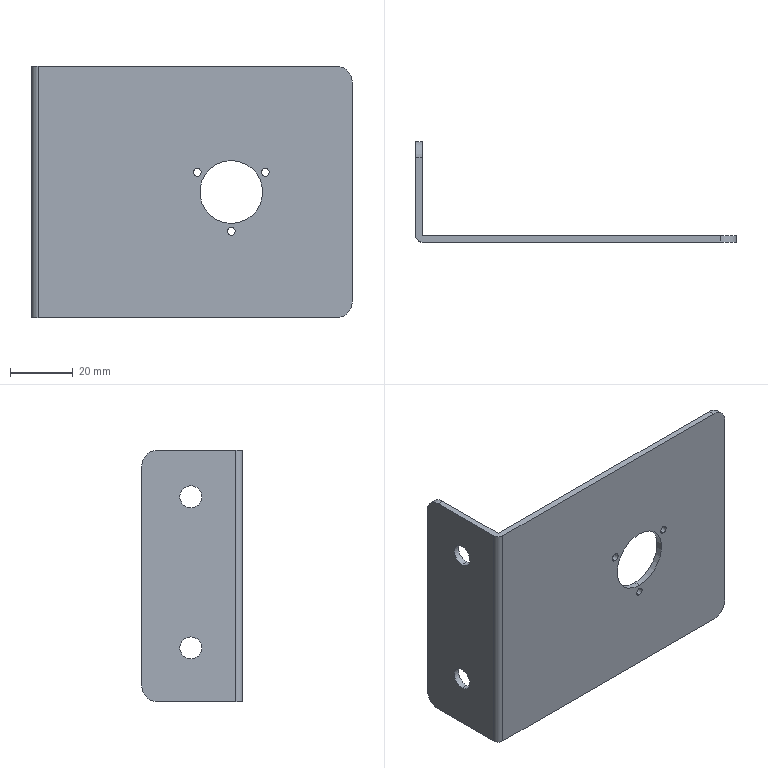Part | STEP file | 400v80 Rear Panel Filler Piece | 1 solid | 26 faces | box 102 x 32 x 80 mm | volume 20190 mm3 | cylinder 18 | plane 8 | commonest cylinder face diameters 2.5 x6 7 x4 10 x4 20 x2 0.2 x1 4.2 x1
STEP:
#1=CARTESIAN_POINT('',(39.258,-59.578,50.));
#2=VERTEX_POINT('',#1);
#3=CARTESIAN_POINT('',(39.258,-59.578,30.));
#4=VERTEX_POINT('',#3);
#5=CARTESIAN_POINT('',(39.258,-59.578,40.));
#6=DIRECTION('',(0.,-1.,0.));
#7=DIRECTION('',(0.,0.,1.));
#8=AXIS2_PLACEMENT_3D('',#5,#6,#7);
#9=CIRCLE('',#8,10.);
#10=EDGE_CURVE('',#2,#4,#9,.T.);
#11=ORIENTED_EDGE('',*,*,#10,.T.);
#12=CARTESIAN_POINT('',(39.258,-57.578,30.));
#13=VERTEX_POINT('',#12);
#14=CARTESIAN_POINT('',(39.258,-67.578,30.));
#15=DIRECTION('',(0.,1.,0.));
#16=VECTOR('',#15,1000.);
#17=LINE('',#14,#16);
#18=EDGE_CURVE('',#4,#13,#17,.T.);
#19=ORIENTED_EDGE('',*,*,#18,.T.);
#20=CARTESIAN_POINT('',(39.258,-57.578,50.));
#21=VERTEX_POINT('',#20);
#22=CARTESIAN_POINT('',(39.258,-57.578,40.));
#23=DIRECTION('',(0.,-1.,0.));
#24=DIRECTION('',(0.,0.,1.));
#25=AXIS2_PLACEMENT_3D('',#22,#23,#24);
#26=CIRCLE('',#25,10.);
#27=EDGE_CURVE('',#21,#13,#26,.T.);
#28=ORIENTED_EDGE('',*,*,#27,.F.);
#29=CARTESIAN_POINT('',(39.258,-67.578,50.));
#30=DIRECTION('',(0.,1.,0.));
#31=VECTOR('',#30,1000.);
#32=LINE('',#29,#31);
#33=EDGE_CURVE('',#2,#21,#32,.T.);
#34=ORIENTED_EDGE('',*,*,#33,.F.);
#35=EDGE_LOOP('',(#11,#19,#28,#34));
#36=FACE_OUTER_BOUND('',#35,.T.);
#37=CARTESIAN_POINT('',(39.258,-67.578,40.));
#38=DIRECTION('',(0.,1.,0.));
#39=DIRECTION('',(0.,0.,1.));
#40=AXIS2_PLACEMENT_3D('',#37,#38,#39);
#41=CYLINDRICAL_SURFACE('',#40,10.);
#42=ADVANCED_FACE('',(#36),#41,.F.);
#43=CARTESIAN_POINT('',(39.258,-59.578,28.75));
#44=VERTEX_POINT('',#43);
#45=CARTESIAN_POINT('',(39.258,-59.578,26.25));
#46=VERTEX_POINT('',#45);
#47=CARTESIAN_POINT('',(39.258,-59.578,27.5));
#48=DIRECTION('',(0.,-1.,0.));
#49=DIRECTION('',(0.,0.,1.));
#50=AXIS2_PLACEMENT_3D('',#47,#48,#49);
#51=CIRCLE('',#50,1.25);
#52=EDGE_CURVE('',#44,#46,#51,.T.);
#53=ORIENTED_EDGE('',*,*,#52,.T.);
#54=CARTESIAN_POINT('',(39.258,-57.578,26.25));
#55=VERTEX_POINT('',#54);
#56=CARTESIAN_POINT('',(39.258,-67.578,26.25));
#57=DIRECTION('',(0.,1.,0.));
#58=VECTOR('',#57,1000.);
#59=LINE('',#56,#58);
#60=EDGE_CURVE('',#46,#55,#59,.T.);
#61=ORIENTED_EDGE('',*,*,#60,.T.);
#62=CARTESIAN_POINT('',(39.258,-57.578,28.75));
#63=VERTEX_POINT('',#62);
#64=CARTESIAN_POINT('',(39.258,-57.578,27.5));
#65=DIRECTION('',(0.,-1.,0.));
#66=DIRECTION('',(0.,0.,1.));
#67=AXIS2_PLACEMENT_3D('',#64,#65,#66);
#68=CIRCLE('',#67,1.25);
#69=EDGE_CURVE('',#63,#55,#68,.T.);
#70=ORIENTED_EDGE('',*,*,#69,.F.);
#71=CARTESIAN_POINT('',(39.258,-67.578,28.75));
#72=DIRECTION('',(0.,1.,0.));
#73=VECTOR('',#72,1000.);
#74=LINE('',#71,#73);
#75=EDGE_CURVE('',#44,#63,#74,.T.);
#76=ORIENTED_EDGE('',*,*,#75,.F.);
#77=EDGE_LOOP('',(#53,#61,#70,#76));
#78=FACE_OUTER_BOUND('',#77,.T.);
#79=CARTESIAN_POINT('',(39.258,-67.578,27.5));
#80=DIRECTION('',(0.,1.,0.));
#81=DIRECTION('',(0.,0.,1.));
#82=AXIS2_PLACEMENT_3D('',#79,#80,#81);
#83=CYLINDRICAL_SURFACE('',#82,1.25);
#84=ADVANCED_FACE('',(#78),#83,.F.);
#85=CARTESIAN_POINT('',(50.084,-59.578,47.5));
#86=VERTEX_POINT('',#85);
#87=CARTESIAN_POINT('',(50.084,-59.578,45.));
#88=VERTEX_POINT('',#87);
#89=CARTESIAN_POINT('',(50.084,-59.578,46.25));
#90=DIRECTION('',(0.,-1.,0.));
#91=DIRECTION('',(0.,0.,1.));
#92=AXIS2_PLACEMENT_3D('',#89,#90,#91);
#93=CIRCLE('',#92,1.25);
#94=EDGE_CURVE('',#86,#88,#93,.T.);
#95=ORIENTED_EDGE('',*,*,#94,.T.);
#96=CARTESIAN_POINT('',(50.084,-57.578,45.));
#97=VERTEX_POINT('',#96);
#98=CARTESIAN_POINT('',(50.084,-67.578,45.));
#99=DIRECTION('',(0.,1.,0.));
#100=VECTOR('',#99,1000.);
#101=LINE('',#98,#100);
#102=EDGE_CURVE('',#88,#97,#101,.T.);
#103=ORIENTED_EDGE('',*,*,#102,.T.);
#104=CARTESIAN_POINT('',(50.084,-57.578,47.5));
#105=VERTEX_POINT('',#104);
#106=CARTESIAN_POINT('',(50.084,-57.578,46.25));
#107=DIRECTION('',(0.,-1.,0.));
#108=DIRECTION('',(0.,0.,1.));
#109=AXIS2_PLACEMENT_3D('',#106,#107,#108);
#110=CIRCLE('',#109,1.25);
#111=EDGE_CURVE('',#105,#97,#110,.T.);
#112=ORIENTED_EDGE('',*,*,#111,.F.);
#113=CARTESIAN_POINT('',(50.084,-67.578,47.5));
#114=DIRECTION('',(0.,1.,0.));
#115=VECTOR('',#114,1000.);
#116=LINE('',#113,#115);
#117=EDGE_CURVE('',#86,#105,#116,.T.);
#118=ORIENTED_EDGE('',*,*,#117,.F.);
#119=EDGE_LOOP('',(#95,#103,#112,#118));
#120=FACE_OUTER_BOUND('',#119,.T.);
#121=CARTESIAN_POINT('',(50.084,-67.578,46.25));
#122=DIRECTION('',(0.,1.,0.));
#123=DIRECTION('',(0.,0.,1.));
#124=AXIS2_PLACEMENT_3D('',#121,#122,#123);
#125=CYLINDRICAL_SURFACE('',#124,1.25);
#126=ADVANCED_FACE('',(#120),#125,.F.);
#127=CARTESIAN_POINT('',(28.433,-59.578,47.5));
#128=VERTEX_POINT('',#127);
#129=CARTESIAN_POINT('',(28.433,-59.578,45.));
#130=VERTEX_POINT('',#129);
#131=CARTESIAN_POINT('',(28.433,-59.578,46.25));
#132=DIRECTION('',(0.,-1.,0.));
#133=DIRECTION('',(0.,0.,1.));
#134=AXIS2_PLACEMENT_3D('',#131,#132,#133);
#135=CIRCLE('',#134,1.25);
#136=EDGE_CURVE('',#128,#130,#135,.T.);
#137=ORIENTED_EDGE('',*,*,#136,.T.);
#138=CARTESIAN_POINT('',(28.433,-57.578,45.));
#139=VERTEX_POINT('',#138);
#140=CARTESIAN_POINT('',(28.433,-67.578,45.));
#141=DIRECTION('',(0.,1.,0.));
#142=VECTOR('',#141,1000.);
#143=LINE('',#140,#142);
#144=EDGE_CURVE('',#130,#139,#143,.T.);
#145=ORIENTED_EDGE('',*,*,#144,.T.);
#146=CARTESIAN_POINT('',(28.433,-57.578,47.5));
#147=VERTEX_POINT('',#146);
#148=CARTESIAN_POINT('',(28.433,-57.578,46.25));
#149=DIRECTION('',(0.,-1.,0.));
#150=DIRECTION('',(0.,0.,1.));
#151=AXIS2_PLACEMENT_3D('',#148,#149,#150);
#152=CIRCLE('',#151,1.25);
#153=EDGE_CURVE('',#147,#139,#152,.T.);
#154=ORIENTED_EDGE('',*,*,#153,.F.);
#155=CARTESIAN_POINT('',(28.433,-67.578,47.5));
#156=DIRECTION('',(0.,1.,0.));
#157=VECTOR('',#156,1000.);
#158=LINE('',#155,#157);
#159=EDGE_CURVE('',#128,#147,#158,.T.);
#160=ORIENTED_EDGE('',*,*,#159,.F.);
#161=EDGE_LOOP('',(#137,#145,#154,#160));
#162=FACE_OUTER_BOUND('',#161,.T.);
#163=CARTESIAN_POINT('',(28.433,-67.578,46.25));
#164=DIRECTION('',(0.,1.,0.));
#165=DIRECTION('',(0.,0.,1.));
#166=AXIS2_PLACEMENT_3D('',#163,#164,#165);
#167=CYLINDRICAL_SURFACE('',#166,1.25);
#168=ADVANCED_FACE('',(#162),#167,.F.);
#169=CARTESIAN_POINT('',(-24.244,-43.225,61.712));
#170=VERTEX_POINT('',#169);
#171=CARTESIAN_POINT('',(-24.244,-43.225,68.712));
#172=VERTEX_POINT('',#171);
#173=CARTESIAN_POINT('',(-24.244,-43.225,65.212));
#174=DIRECTION('',(-1.,0.,0.));
#175=DIRECTION('',(0.,0.,-1.));
#176=AXIS2_PLACEMENT_3D('',#173,#174,#175);
#177=CIRCLE('',#176,3.5);
#178=EDGE_CURVE('',#170,#172,#177,.T.);
#179=ORIENTED_EDGE('',*,*,#178,.T.);
#180=CARTESIAN_POINT('',(-22.244,-43.225,68.712));
#181=VERTEX_POINT('',#180);
#182=CARTESIAN_POINT('',(-32.244,-43.225,68.712));
#183=DIRECTION('',(1.,0.,0.));
#184=VECTOR('',#183,1000.);
#185=LINE('',#182,#184);
#186=EDGE_CURVE('',#172,#181,#185,.T.);
#187=ORIENTED_EDGE('',*,*,#186,.T.);
#188=CARTESIAN_POINT('',(-22.244,-43.225,61.712));
#189=VERTEX_POINT('',#188);
#190=CARTESIAN_POINT('',(-22.244,-43.225,65.212));
#191=DIRECTION('',(-1.,0.,0.));
#192=DIRECTION('',(0.,0.,-1.));
#193=AXIS2_PLACEMENT_3D('',#190,#191,#192);
#194=CIRCLE('',#193,3.5);
#195=EDGE_CURVE('',#189,#181,#194,.T.);
#196=ORIENTED_EDGE('',*,*,#195,.F.);
#197=CARTESIAN_POINT('',(-32.244,-43.225,61.712));
#198=DIRECTION('',(1.,0.,0.));
#199=VECTOR('',#198,1000.);
#200=LINE('',#197,#199);
#201=EDGE_CURVE('',#170,#189,#200,.T.);
#202=ORIENTED_EDGE('',*,*,#201,.F.);
#203=EDGE_LOOP('',(#179,#187,#196,#202));
#204=FACE_OUTER_BOUND('',#203,.T.);
#205=CARTESIAN_POINT('',(-32.244,-43.225,65.212));
#206=DIRECTION('',(1.,0.,0.));
#207=DIRECTION('',(0.,0.,-1.));
#208=AXIS2_PLACEMENT_3D('',#205,#206,#207);
#209=CYLINDRICAL_SURFACE('',#208,3.5);
#210=ADVANCED_FACE('',(#204),#209,.F.);
#211=CARTESIAN_POINT('',(-24.244,-43.225,13.607));
#212=VERTEX_POINT('',#211);
#213=CARTESIAN_POINT('',(-24.244,-43.225,20.607));
#214=VERTEX_POINT('',#213);
#215=CARTESIAN_POINT('',(-24.244,-43.225,17.107));
#216=DIRECTION('',(-1.,0.,0.));
#217=DIRECTION('',(0.,0.,-1.));
#218=AXIS2_PLACEMENT_3D('',#215,#216,#217);
#219=CIRCLE('',#218,3.5);
#220=EDGE_CURVE('',#212,#214,#219,.T.);
#221=ORIENTED_EDGE('',*,*,#220,.T.);
#222=CARTESIAN_POINT('',(-22.244,-43.225,20.607));
#223=VERTEX_POINT('',#222);
#224=CARTESIAN_POINT('',(-32.244,-43.225,20.607));
#225=DIRECTION('',(1.,0.,0.));
#226=VECTOR('',#225,1000.);
#227=LINE('',#224,#226);
#228=EDGE_CURVE('',#214,#223,#227,.T.);
#229=ORIENTED_EDGE('',*,*,#228,.T.);
#230=CARTESIAN_POINT('',(-22.244,-43.225,13.607));
#231=VERTEX_POINT('',#230);
#232=CARTESIAN_POINT('',(-22.244,-43.225,17.107));
#233=DIRECTION('',(-1.,0.,0.));
#234=DIRECTION('',(0.,0.,-1.));
#235=AXIS2_PLACEMENT_3D('',#232,#233,#234);
#236=CIRCLE('',#235,3.5);
#237=EDGE_CURVE('',#231,#223,#236,.T.);
#238=ORIENTED_EDGE('',*,*,#237,.F.);
#239=CARTESIAN_POINT('',(-32.244,-43.225,13.607));
#240=DIRECTION('',(1.,0.,0.));
#241=VECTOR('',#240,1000.);
#242=LINE('',#239,#241);
#243=EDGE_CURVE('',#212,#231,#242,.T.);
#244=ORIENTED_EDGE('',*,*,#243,.F.);
#245=EDGE_LOOP('',(#221,#229,#238,#244));
#246=FACE_OUTER_BOUND('',#245,.T.);
#247=CARTESIAN_POINT('',(-32.244,-43.225,17.107));
#248=DIRECTION('',(1.,0.,0.));
#249=DIRECTION('',(0.,0.,-1.));
#250=AXIS2_PLACEMENT_3D('',#247,#248,#249);
#251=CYLINDRICAL_SURFACE('',#250,3.5);
#252=ADVANCED_FACE('',(#246),#251,.F.);
#253=CARTESIAN_POINT('',(77.756,-59.578,5.));
#254=VERTEX_POINT('',#253);
#255=CARTESIAN_POINT('',(72.756,-59.578,0.));
#256=VERTEX_POINT('',#255);
#257=CARTESIAN_POINT('',(72.756,-59.578,5.));
#258=DIRECTION('',(0.,1.,0.));
#259=DIRECTION('',(0.,0.,-1.));
#260=AXIS2_PLACEMENT_3D('',#257,#258,#259);
#261=CIRCLE('',#260,5.);
#262=EDGE_CURVE('',#254,#256,#261,.T.);
#263=ORIENTED_EDGE('',*,*,#262,.F.);
#264=CARTESIAN_POINT('',(77.756,-59.578,75.));
#265=VERTEX_POINT('',#264);
#266=CARTESIAN_POINT('',(77.756,-59.578,80.));
#267=DIRECTION('',(0.,0.,-1.));
#268=VECTOR('',#267,1000.);
#269=LINE('',#266,#268);
#270=EDGE_CURVE('',#265,#254,#269,.T.);
#271=ORIENTED_EDGE('',*,*,#270,.F.);
#272=CARTESIAN_POINT('',(72.756,-59.578,80.));
#273=VERTEX_POINT('',#272);
#274=CARTESIAN_POINT('',(72.756,-59.578,75.));
#275=DIRECTION('',(0.,1.,0.));
#276=DIRECTION('',(0.,0.,-1.));
#277=AXIS2_PLACEMENT_3D('',#274,#275,#276);
#278=CIRCLE('',#277,5.);
#279=EDGE_CURVE('',#273,#265,#278,.T.);
#280=ORIENTED_EDGE('',*,*,#279,.F.);
#281=CARTESIAN_POINT('',(-22.144,-59.578,80.));
#282=VERTEX_POINT('',#281);
#283=CARTESIAN_POINT('',(-22.244,-59.578,80.));
#284=DIRECTION('',(1.,0.,0.));
#285=VECTOR('',#284,1000.);
#286=LINE('',#283,#285);
#287=EDGE_CURVE('',#282,#273,#286,.T.);
#288=ORIENTED_EDGE('',*,*,#287,.F.);
#289=CARTESIAN_POINT('',(-22.144,-59.578,0.));
#290=VERTEX_POINT('',#289);
#291=CARTESIAN_POINT('',(-22.144,-59.578,80.));
#292=DIRECTION('',(0.,0.,1.));
#293=VECTOR('',#292,1000.);
#294=LINE('',#291,#293);
#295=EDGE_CURVE('',#290,#282,#294,.T.);
#296=ORIENTED_EDGE('',*,*,#295,.F.);
#297=CARTESIAN_POINT('',(-22.244,-59.578,0.));
#298=DIRECTION('',(-1.,0.,0.));
#299=VECTOR('',#298,1000.);
#300=LINE('',#297,#299);
#301=EDGE_CURVE('',#256,#290,#300,.T.);
#302=ORIENTED_EDGE('',*,*,#301,.F.);
#303=EDGE_LOOP('',(#263,#271,#280,#288,#296,#302));
#304=FACE_OUTER_BOUND('',#303,.T.);
#305=ORIENTED_EDGE('',*,*,#10,.F.);
#306=CARTESIAN_POINT('',(39.258,-59.578,40.));
#307=DIRECTION('',(0.,-1.,0.));
#308=DIRECTION('',(0.,0.,1.));
#309=AXIS2_PLACEMENT_3D('',#306,#307,#308);
#310=CIRCLE('',#309,10.);
#311=EDGE_CURVE('',#4,#2,#310,.T.);
#312=ORIENTED_EDGE('',*,*,#311,.F.);
#313=EDGE_LOOP('',(#305,#312));
#314=FACE_BOUND('',#313,.T.);
#315=ORIENTED_EDGE('',*,*,#52,.F.);
#316=CARTESIAN_POINT('',(39.258,-59.578,27.5));
#317=DIRECTION('',(0.,-1.,0.));
#318=DIRECTION('',(0.,0.,1.));
#319=AXIS2_PLACEMENT_3D('',#316,#317,#318);
#320=CIRCLE('',#319,1.25);
#321=EDGE_CURVE('',#46,#44,#320,.T.);
#322=ORIENTED_EDGE('',*,*,#321,.F.);
#323=EDGE_LOOP('',(#315,#322));
#324=FACE_BOUND('',#323,.T.);
#325=ORIENTED_EDGE('',*,*,#94,.F.);
#326=CARTESIAN_POINT('',(50.084,-59.578,46.25));
#327=DIRECTION('',(0.,-1.,0.));
#328=DIRECTION('',(0.,0.,1.));
#329=AXIS2_PLACEMENT_3D('',#326,#327,#328);
#330=CIRCLE('',#329,1.25);
#331=EDGE_CURVE('',#88,#86,#330,.T.);
#332=ORIENTED_EDGE('',*,*,#331,.F.);
#333=EDGE_LOOP('',(#325,#332));
#334=FACE_BOUND('',#333,.T.);
#335=ORIENTED_EDGE('',*,*,#136,.F.);
#336=CARTESIAN_POINT('',(28.433,-59.578,46.25));
#337=DIRECTION('',(0.,-1.,0.));
#338=DIRECTION('',(0.,0.,1.));
#339=AXIS2_PLACEMENT_3D('',#336,#337,#338);
#340=CIRCLE('',#339,1.25);
#341=EDGE_CURVE('',#130,#128,#340,.T.);
#342=ORIENTED_EDGE('',*,*,#341,.F.);
#343=EDGE_LOOP('',(#335,#342));
#344=FACE_BOUND('',#343,.T.);
#345=CARTESIAN_POINT('',(-22.244,-59.578,80.));
#346=DIRECTION('',(0.,1.,0.));
#347=DIRECTION('',(0.,0.,1.));
#348=AXIS2_PLACEMENT_3D('',#345,#346,#347);
#349=PLANE('',#348);
#350=ADVANCED_FACE('',(#304,#314,#324,#334,#344),#349,.F.);
#351=ORIENTED_EDGE('',*,*,#301,.T.);
#352=CARTESIAN_POINT('',(-24.244,-57.478,0.));
#353=VERTEX_POINT('',#352);
#354=CARTESIAN_POINT('',(-22.144,-57.478,0.));
#355=DIRECTION('',(0.,0.,1.));
#356=DIRECTION('',(-1.,0.,0.));
#357=AXIS2_PLACEMENT_3D('',#354,#355,#356);
#358=CIRCLE('',#357,2.1);
#359=EDGE_CURVE('',#353,#290,#358,.T.);
#360=ORIENTED_EDGE('',*,*,#359,.F.);
#361=CARTESIAN_POINT('',(-24.244,-32.578,0.));
#362=VERTEX_POINT('',#361);
#363=CARTESIAN_POINT('',(-24.244,-27.578,0.));
#364=DIRECTION('',(0.,1.,0.));
#365=VECTOR('',#364,1000.);
#366=LINE('',#363,#365);
#367=EDGE_CURVE('',#353,#362,#366,.T.);
#368=ORIENTED_EDGE('',*,*,#367,.T.);
#369=CARTESIAN_POINT('',(-22.244,-32.578,0.));
#370=VERTEX_POINT('',#369);
#371=CARTESIAN_POINT('',(-22.144,-32.578,0.));
#372=DIRECTION('',(1.,0.,0.));
#373=VECTOR('',#372,1000.);
#374=LINE('',#371,#373);
#375=EDGE_CURVE('',#362,#370,#374,.T.);
#376=ORIENTED_EDGE('',*,*,#375,.T.);
#377=CARTESIAN_POINT('',(-22.244,-57.478,0.));
#378=VERTEX_POINT('',#377);
#379=CARTESIAN_POINT('',(-22.244,-59.578,0.));
#380=DIRECTION('',(0.,-1.,0.));
#381=VECTOR('',#380,1000.);
#382=LINE('',#379,#381);
#383=EDGE_CURVE('',#370,#378,#382,.T.);
#384=ORIENTED_EDGE('',*,*,#383,.T.);
#385=CARTESIAN_POINT('',(-22.144,-57.578,0.));
#386=VERTEX_POINT('',#385);
#387=CARTESIAN_POINT('',(-22.144,-57.478,0.));
#388=DIRECTION('',(0.,0.,1.));
#389=DIRECTION('',(-1.,0.,0.));
#390=AXIS2_PLACEMENT_3D('',#387,#388,#389);
#391=CIRCLE('',#390,0.1);
#392=EDGE_CURVE('',#378,#386,#391,.T.);
#393=ORIENTED_EDGE('',*,*,#392,.T.);
#394=CARTESIAN_POINT('',(72.756,-57.578,0.));
#395=VERTEX_POINT('',#394);
#396=CARTESIAN_POINT('',(-22.144,-57.578,0.));
#397=DIRECTION('',(1.,0.,0.));
#398=VECTOR('',#397,1000.);
#399=LINE('',#396,#398);
#400=EDGE_CURVE('',#386,#395,#399,.T.);
#401=ORIENTED_EDGE('',*,*,#400,.T.);
#402=CARTESIAN_POINT('',(72.756,-57.478,0.));
#403=DIRECTION('',(0.,-1.,0.));
#404=VECTOR('',#403,1000.);
#405=LINE('',#402,#404);
#406=EDGE_CURVE('',#395,#256,#405,.T.);
#407=ORIENTED_EDGE('',*,*,#406,.T.);
#408=EDGE_LOOP('',(#351,#360,#368,#376,#384,#393,#401,#407));
#409=FACE_OUTER_BOUND('',#408,.T.);
#410=CARTESIAN_POINT('',(-22.144,-57.478,0.));
#411=DIRECTION('',(0.,0.,-1.));
#412=DIRECTION('',(-1.,0.,0.));
#413=AXIS2_PLACEMENT_3D('',#410,#411,#412);
#414=PLANE('',#413);
#415=ADVANCED_FACE('',(#409),#414,.T.);
#416=ORIENTED_EDGE('',*,*,#262,.T.);
#417=ORIENTED_EDGE('',*,*,#406,.F.);
#418=CARTESIAN_POINT('',(77.756,-57.578,5.));
#419=VERTEX_POINT('',#418);
#420=CARTESIAN_POINT('',(72.756,-57.578,5.));
#421=DIRECTION('',(0.,-1.,0.));
#422=DIRECTION('',(0.,0.,-1.));
#423=AXIS2_PLACEMENT_3D('',#420,#421,#422);
#424=CIRCLE('',#423,5.);
#425=EDGE_CURVE('',#395,#419,#424,.T.);
#426=ORIENTED_EDGE('',*,*,#425,.T.);
#427=CARTESIAN_POINT('',(77.756,-57.478,5.));
#428=DIRECTION('',(0.,-1.,0.));
#429=VECTOR('',#428,1000.);
#430=LINE('',#427,#429);
#431=EDGE_CURVE('',#419,#254,#430,.T.);
#432=ORIENTED_EDGE('',*,*,#431,.T.);
#433=EDGE_LOOP('',(#416,#417,#426,#432));
#434=FACE_OUTER_BOUND('',#433,.T.);
#435=CARTESIAN_POINT('',(72.756,-57.478,5.));
#436=DIRECTION('',(0.,-1.,0.));
#437=DIRECTION('',(0.,0.,-1.));
#438=AXIS2_PLACEMENT_3D('',#435,#436,#437);
#439=CYLINDRICAL_SURFACE('',#438,5.);
#440=ADVANCED_FACE('',(#434),#439,.T.);
#441=CARTESIAN_POINT('',(77.756,-57.578,75.));
#442=VERTEX_POINT('',#441);
#443=CARTESIAN_POINT('',(77.756,-57.578,80.));
#444=DIRECTION('',(0.,0.,1.));
#445=VECTOR('',#444,1000.);
#446=LINE('',#443,#445);
#447=EDGE_CURVE('',#419,#442,#446,.T.);
#448=ORIENTED_EDGE('',*,*,#447,.T.);
#449=CARTESIAN_POINT('',(77.756,-57.578,75.));
#450=DIRECTION('',(0.,-1.,0.));
#451=VECTOR('',#450,1000.);
#452=LINE('',#449,#451);
#453=EDGE_CURVE('',#442,#265,#452,.T.);
#454=ORIENTED_EDGE('',*,*,#453,.T.);
#455=ORIENTED_EDGE('',*,*,#270,.T.);
#456=ORIENTED_EDGE('',*,*,#431,.F.);
#457=EDGE_LOOP('',(#448,#454,#455,#456));
#458=FACE_OUTER_BOUND('',#457,.T.);
#459=CARTESIAN_POINT('',(77.756,-57.578,80.));
#460=DIRECTION('',(1.,0.,0.));
#461=DIRECTION('',(0.,0.,-1.));
#462=AXIS2_PLACEMENT_3D('',#459,#460,#461);
#463=PLANE('',#462);
#464=ADVANCED_FACE('',(#458),#463,.T.);
#465=ORIENTED_EDGE('',*,*,#279,.T.);
#466=ORIENTED_EDGE('',*,*,#453,.F.);
#467=CARTESIAN_POINT('',(72.756,-57.578,80.));
#468=VERTEX_POINT('',#467);
#469=CARTESIAN_POINT('',(72.756,-57.578,75.));
#470=DIRECTION('',(0.,-1.,0.));
#471=DIRECTION('',(0.,0.,-1.));
#472=AXIS2_PLACEMENT_3D('',#469,#470,#471);
#473=CIRCLE('',#472,5.);
#474=EDGE_CURVE('',#442,#468,#473,.T.);
#475=ORIENTED_EDGE('',*,*,#474,.T.);
#476=CARTESIAN_POINT('',(72.756,-57.578,80.));
#477=DIRECTION('',(0.,-1.,0.));
#478=VECTOR('',#477,1000.);
#479=LINE('',#476,#478);
#480=EDGE_CURVE('',#468,#273,#479,.T.);
#481=ORIENTED_EDGE('',*,*,#480,.T.);
#482=EDGE_LOOP('',(#465,#466,#475,#481));
#483=FACE_OUTER_BOUND('',#482,.T.);
#484=CARTESIAN_POINT('',(72.756,-57.578,75.));
#485=DIRECTION('',(0.,-1.,0.));
#486=DIRECTION('',(0.,0.,-1.));
#487=AXIS2_PLACEMENT_3D('',#484,#485,#486);
#488=CYLINDRICAL_SURFACE('',#487,5.);
#489=ADVANCED_FACE('',(#483),#488,.T.);
#490=CARTESIAN_POINT('',(-22.144,-57.578,80.));
#491=VERTEX_POINT('',#490);
#492=CARTESIAN_POINT('',(-24.244,-57.578,80.));
#493=DIRECTION('',(-1.,0.,0.));
#494=VECTOR('',#493,1000.);
#495=LINE('',#492,#494);
#496=EDGE_CURVE('',#468,#491,#495,.T.);
#497=ORIENTED_EDGE('',*,*,#496,.T.);
#498=CARTESIAN_POINT('',(-22.244,-57.478,80.));
#499=VERTEX_POINT('',#498);
#500=CARTESIAN_POINT('',(-22.144,-57.478,80.));
#501=DIRECTION('',(0.,0.,-1.));
#502=DIRECTION('',(-1.,0.,0.));
#503=AXIS2_PLACEMENT_3D('',#500,#501,#502);
#504=CIRCLE('',#503,0.1);
#505=EDGE_CURVE('',#491,#499,#504,.T.);
#506=ORIENTED_EDGE('',*,*,#505,.T.);
#507=CARTESIAN_POINT('',(-22.244,-32.578,80.));
#508=VERTEX_POINT('',#507);
#509=CARTESIAN_POINT('',(-22.244,-57.478,80.));
#510=DIRECTION('',(0.,-1.,0.));
#511=VECTOR('',#510,1000.);
#512=LINE('',#509,#511);
#513=EDGE_CURVE('',#508,#499,#512,.T.);
#514=ORIENTED_EDGE('',*,*,#513,.F.);
#515=CARTESIAN_POINT('',(-24.244,-32.578,80.));
#516=VERTEX_POINT('',#515);
#517=CARTESIAN_POINT('',(-22.144,-32.578,80.));
#518=DIRECTION('',(1.,0.,0.));
#519=VECTOR('',#518,1000.);
#520=LINE('',#517,#519);
#521=EDGE_CURVE('',#516,#508,#520,.T.);
#522=ORIENTED_EDGE('',*,*,#521,.F.);
#523=CARTESIAN_POINT('',(-24.244,-57.478,80.));
#524=VERTEX_POINT('',#523);
#525=CARTESIAN_POINT('',(-24.244,-27.578,80.));
#526=DIRECTION('',(0.,-1.,0.));
#527=VECTOR('',#526,1000.);
#528=LINE('',#525,#527);
#529=EDGE_CURVE('',#516,#524,#528,.T.);
#530=ORIENTED_EDGE('',*,*,#529,.T.);
#531=CARTESIAN_POINT('',(-22.144,-57.478,80.));
#532=DIRECTION('',(0.,0.,-1.));
#533=DIRECTION('',(-1.,0.,0.));
#534=AXIS2_PLACEMENT_3D('',#531,#532,#533);
#535=CIRCLE('',#534,2.1);
#536=EDGE_CURVE('',#282,#524,#535,.T.);
#537=ORIENTED_EDGE('',*,*,#536,.F.);
#538=ORIENTED_EDGE('',*,*,#287,.T.);
#539=ORIENTED_EDGE('',*,*,#480,.F.);
#540=EDGE_LOOP('',(#497,#506,#514,#522,#530,#537,#538,#539));
#541=FACE_OUTER_BOUND('',#540,.T.);
#542=CARTESIAN_POINT('',(-24.244,-57.478,80.));
#543=DIRECTION('',(0.,0.,1.));
#544=DIRECTION('',(1.,0.,0.));
#545=AXIS2_PLACEMENT_3D('',#542,#543,#544);
#546=PLANE('',#545);
#547=ADVANCED_FACE('',(#541),#546,.T.);
#548=ORIENTED_EDGE('',*,*,#536,.T.);
#549=CARTESIAN_POINT('',(-24.244,-57.478,80.));
#550=DIRECTION('',(0.,0.,-1.));
#551=VECTOR('',#550,1000.);
#552=LINE('',#549,#551);
#553=EDGE_CURVE('',#524,#353,#552,.T.);
#554=ORIENTED_EDGE('',*,*,#553,.T.);
#555=ORIENTED_EDGE('',*,*,#359,.T.);
#556=ORIENTED_EDGE('',*,*,#295,.T.);
#557=EDGE_LOOP('',(#548,#554,#555,#556));
#558=FACE_OUTER_BOUND('',#557,.T.);
#559=CARTESIAN_POINT('',(-22.144,-57.478,80.));
#560=DIRECTION('',(0.,0.,-1.));
#561=DIRECTION('',(-1.,0.,0.));
#562=AXIS2_PLACEMENT_3D('',#559,#560,#561);
#563=CYLINDRICAL_SURFACE('',#562,2.1);
#564=ADVANCED_FACE('',(#558),#563,.T.);
#565=ORIENTED_EDGE('',*,*,#18,.F.);
#566=ORIENTED_EDGE('',*,*,#311,.T.);
#567=ORIENTED_EDGE('',*,*,#33,.T.);
#568=CARTESIAN_POINT('',(39.258,-57.578,40.));
#569=DIRECTION('',(0.,-1.,0.));
#570=DIRECTION('',(0.,0.,1.));
#571=AXIS2_PLACEMENT_3D('',#568,#569,#570);
#572=CIRCLE('',#571,10.);
#573=EDGE_CURVE('',#13,#21,#572,.T.);
#574=ORIENTED_EDGE('',*,*,#573,.F.);
#575=EDGE_LOOP('',(#565,#566,#567,#574));
#576=FACE_OUTER_BOUND('',#575,.T.);
#577=CARTESIAN_POINT('',(39.258,-67.578,40.));
#578=DIRECTION('',(0.,1.,0.));
#579=DIRECTION('',(0.,0.,1.));
#580=AXIS2_PLACEMENT_3D('',#577,#578,#579);
#581=CYLINDRICAL_SURFACE('',#580,10.);
#582=ADVANCED_FACE('',(#576),#581,.F.);
#583=ORIENTED_EDGE('',*,*,#60,.F.);
#584=ORIENTED_EDGE('',*,*,#321,.T.);
#585=ORIENTED_EDGE('',*,*,#75,.T.);
#586=CARTESIAN_POINT('',(39.258,-57.578,27.5));
#587=DIRECTION('',(0.,-1.,0.));
#588=DIRECTION('',(0.,0.,1.));
#589=AXIS2_PLACEMENT_3D('',#586,#587,#588);
#590=CIRCLE('',#589,1.25);
#591=EDGE_CURVE('',#55,#63,#590,.T.);
#592=ORIENTED_EDGE('',*,*,#591,.F.);
#593=EDGE_LOOP('',(#583,#584,#585,#592));
#594=FACE_OUTER_BOUND('',#593,.T.);
#595=CARTESIAN_POINT('',(39.258,-67.578,27.5));
#596=DIRECTION('',(0.,1.,0.));
#597=DIRECTION('',(0.,0.,1.));
#598=AXIS2_PLACEMENT_3D('',#595,#596,#597);
#599=CYLINDRICAL_SURFACE('',#598,1.25);
#600=ADVANCED_FACE('',(#594),#599,.F.);
#601=ORIENTED_EDGE('',*,*,#102,.F.);
#602=ORIENTED_EDGE('',*,*,#331,.T.);
#603=ORIENTED_EDGE('',*,*,#117,.T.);
#604=CARTESIAN_POINT('',(50.084,-57.578,46.25));
#605=DIRECTION('',(0.,-1.,0.));
#606=DIRECTION('',(0.,0.,1.));
#607=AXIS2_PLACEMENT_3D('',#604,#605,#606);
#608=CIRCLE('',#607,1.25);
#609=EDGE_CURVE('',#97,#105,#608,.T.);
#610=ORIENTED_EDGE('',*,*,#609,.F.);
#611=EDGE_LOOP('',(#601,#602,#603,#610));
#612=FACE_OUTER_BOUND('',#611,.T.);
#613=CARTESIAN_POINT('',(50.084,-67.578,46.25));
#614=DIRECTION('',(0.,1.,0.));
#615=DIRECTION('',(0.,0.,1.));
#616=AXIS2_PLACEMENT_3D('',#613,#614,#615);
#617=CYLINDRICAL_SURFACE('',#616,1.25);
#618=ADVANCED_FACE('',(#612),#617,.F.);
#619=ORIENTED_EDGE('',*,*,#144,.F.);
#620=ORIENTED_EDGE('',*,*,#341,.T.);
#621=ORIENTED_EDGE('',*,*,#159,.T.);
#622=CARTESIAN_POINT('',(28.433,-57.578,46.25));
#623=DIRECTION('',(0.,-1.,0.));
#624=DIRECTION('',(0.,0.,1.));
#625=AXIS2_PLACEMENT_3D('',#622,#623,#624);
#626=CIRCLE('',#625,1.25);
#627=EDGE_CURVE('',#139,#147,#626,.T.);
#628=ORIENTED_EDGE('',*,*,#627,.F.);
#629=EDGE_LOOP('',(#619,#620,#621,#628));
#630=FACE_OUTER_BOUND('',#629,.T.);
#631=CARTESIAN_POINT('',(28.433,-67.578,46.25));
#632=DIRECTION('',(0.,1.,0.));
#633=DIRECTION('',(0.,0.,1.));
#634=AXIS2_PLACEMENT_3D('',#631,#632,#633);
#635=CYLINDRICAL_SURFACE('',#634,1.25);
#636=ADVANCED_FACE('',(#630),#635,.F.);
#637=ORIENTED_EDGE('',*,*,#496,.F.);
#638=ORIENTED_EDGE('',*,*,#474,.F.);
#639=ORIENTED_EDGE('',*,*,#447,.F.);
#640=ORIENTED_EDGE('',*,*,#425,.F.);
#641=ORIENTED_EDGE('',*,*,#400,.F.);
#642=CARTESIAN_POINT('',(-22.144,-57.578,80.));
#643=DIRECTION('',(0.,0.,1.));
#644=VECTOR('',#643,1000.);
#645=LINE('',#642,#644);
#646=EDGE_CURVE('',#386,#491,#645,.T.);
#647=ORIENTED_EDGE('',*,*,#646,.T.);
#648=EDGE_LOOP('',(#637,#638,#639,#640,#641,#647));
#649=FACE_OUTER_BOUND('',#648,.T.);
#650=ORIENTED_EDGE('',*,*,#27,.T.);
#651=ORIENTED_EDGE('',*,*,#573,.T.);
#652=EDGE_LOOP('',(#650,#651));
#653=FACE_BOUND('',#652,.T.);
#654=ORIENTED_EDGE('',*,*,#69,.T.);
#655=ORIENTED_EDGE('',*,*,#591,.T.);
#656=EDGE_LOOP('',(#654,#655));
#657=FACE_BOUND('',#656,.T.);
#658=ORIENTED_EDGE('',*,*,#111,.T.);
#659=ORIENTED_EDGE('',*,*,#609,.T.);
#660=EDGE_LOOP('',(#658,#659));
#661=FACE_BOUND('',#660,.T.);
#662=ORIENTED_EDGE('',*,*,#153,.T.);
#663=ORIENTED_EDGE('',*,*,#627,.T.);
#664=EDGE_LOOP('',(#662,#663));
#665=FACE_BOUND('',#664,.T.);
#666=CARTESIAN_POINT('',(-22.244,-57.578,80.));
#667=DIRECTION('',(0.,1.,0.));
#668=DIRECTION('',(0.,0.,1.));
#669=AXIS2_PLACEMENT_3D('',#666,#667,#668);
#670=PLANE('',#669);
#671=ADVANCED_FACE('',(#649,#653,#657,#661,#665),#670,.T.);
#672=CARTESIAN_POINT('',(-24.244,-27.578,75.));
#673=VERTEX_POINT('',#672);
#674=CARTESIAN_POINT('',(-24.244,-32.578,75.));
#675=DIRECTION('',(1.,0.,0.));
#676=DIRECTION('',(0.,0.,1.));
#677=AXIS2_PLACEMENT_3D('',#674,#675,#676);
#678=CIRCLE('',#677,5.);
#679=EDGE_CURVE('',#673,#516,#678,.T.);
#680=ORIENTED_EDGE('',*,*,#679,.F.);
#681=CARTESIAN_POINT('',(-24.244,-27.578,5.));
#682=VERTEX_POINT('',#681);
#683=CARTESIAN_POINT('',(-24.244,-27.578,80.));
#684=DIRECTION('',(0.,0.,1.));
#685=VECTOR('',#684,1000.);
#686=LINE('',#683,#685);
#687=EDGE_CURVE('',#682,#673,#686,.T.);
#688=ORIENTED_EDGE('',*,*,#687,.F.);
#689=CARTESIAN_POINT('',(-24.244,-32.578,5.));
#690=DIRECTION('',(1.,0.,0.));
#691=DIRECTION('',(0.,0.,-1.));
#692=AXIS2_PLACEMENT_3D('',#689,#690,#691);
#693=CIRCLE('',#692,5.);
#694=EDGE_CURVE('',#362,#682,#693,.T.);
#695=ORIENTED_EDGE('',*,*,#694,.F.);
#696=ORIENTED_EDGE('',*,*,#367,.F.);
#697=ORIENTED_EDGE('',*,*,#553,.F.);
#698=ORIENTED_EDGE('',*,*,#529,.F.);
#699=EDGE_LOOP('',(#680,#688,#695,#696,#697,#698));
#700=FACE_OUTER_BOUND('',#699,.T.);
#701=ORIENTED_EDGE('',*,*,#178,.F.);
#702=CARTESIAN_POINT('',(-24.244,-43.225,65.212));
#703=DIRECTION('',(-1.,0.,0.));
#704=DIRECTION('',(0.,0.,-1.));
#705=AXIS2_PLACEMENT_3D('',#702,#703,#704);
#706=CIRCLE('',#705,3.5);
#707=EDGE_CURVE('',#172,#170,#706,.T.);
#708=ORIENTED_EDGE('',*,*,#707,.F.);
#709=EDGE_LOOP('',(#701,#708));
#710=FACE_BOUND('',#709,.T.);
#711=ORIENTED_EDGE('',*,*,#220,.F.);
#712=CARTESIAN_POINT('',(-24.244,-43.225,17.107));
#713=DIRECTION('',(-1.,0.,0.));
#714=DIRECTION('',(0.,0.,-1.));
#715=AXIS2_PLACEMENT_3D('',#712,#713,#714);
#716=CIRCLE('',#715,3.5);
#717=EDGE_CURVE('',#214,#212,#716,.T.);
#718=ORIENTED_EDGE('',*,*,#717,.F.);
#719=EDGE_LOOP('',(#711,#718));
#720=FACE_BOUND('',#719,.T.);
#721=CARTESIAN_POINT('',(-24.244,-27.578,80.));
#722=DIRECTION('',(1.,0.,0.));
#723=DIRECTION('',(0.,0.,-1.));
#724=AXIS2_PLACEMENT_3D('',#721,#722,#723);
#725=PLANE('',#724);
#726=ADVANCED_FACE('',(#700,#710,#720),#725,.F.);
#727=CARTESIAN_POINT('',(-22.244,-57.478,80.));
#728=DIRECTION('',(0.,0.,-1.));
#729=VECTOR('',#728,1000.);
#730=LINE('',#727,#729);
#731=EDGE_CURVE('',#499,#378,#730,.T.);
#732=ORIENTED_EDGE('',*,*,#731,.F.);
#733=ORIENTED_EDGE('',*,*,#505,.F.);
#734=ORIENTED_EDGE('',*,*,#646,.F.);
#735=ORIENTED_EDGE('',*,*,#392,.F.);
#736=EDGE_LOOP('',(#732,#733,#734,#735));
#737=FACE_OUTER_BOUND('',#736,.T.);
#738=CARTESIAN_POINT('',(-22.144,-57.478,80.));
#739=DIRECTION('',(0.,0.,-1.));
#740=DIRECTION('',(-1.,0.,0.));
#741=AXIS2_PLACEMENT_3D('',#738,#739,#740);
#742=CYLINDRICAL_SURFACE('',#741,0.1);
#743=ADVANCED_FACE('',(#737),#742,.F.);
#744=CARTESIAN_POINT('',(-22.244,-27.578,75.));
#745=VERTEX_POINT('',#744);
#746=CARTESIAN_POINT('',(-22.244,-32.578,75.));
#747=DIRECTION('',(-1.,0.,0.));
#748=DIRECTION('',(0.,0.,1.));
#749=AXIS2_PLACEMENT_3D('',#746,#747,#748);
#750=CIRCLE('',#749,5.);
#751=EDGE_CURVE('',#508,#745,#750,.T.);
#752=ORIENTED_EDGE('',*,*,#751,.T.);
#753=CARTESIAN_POINT('',(-24.244,-27.578,75.));
#754=DIRECTION('',(-1.,0.,0.));
#755=VECTOR('',#754,1000.);
#756=LINE('',#753,#755);
#757=EDGE_CURVE('',#745,#673,#756,.T.);
#758=ORIENTED_EDGE('',*,*,#757,.T.);
#759=ORIENTED_EDGE('',*,*,#679,.T.);
#760=ORIENTED_EDGE('',*,*,#521,.T.);
#761=EDGE_LOOP('',(#752,#758,#759,#760));
#762=FACE_OUTER_BOUND('',#761,.T.);
#763=CARTESIAN_POINT('',(-24.244,-32.578,75.));
#764=DIRECTION('',(-1.,0.,0.));
#765=DIRECTION('',(0.,0.,1.));
#766=AXIS2_PLACEMENT_3D('',#763,#764,#765);
#767=CYLINDRICAL_SURFACE('',#766,5.);
#768=ADVANCED_FACE('',(#762),#767,.T.);
#769=CARTESIAN_POINT('',(-22.244,-27.578,5.));
#770=VERTEX_POINT('',#769);
#771=CARTESIAN_POINT('',(-22.244,-27.578,80.));
#772=DIRECTION('',(0.,0.,-1.));
#773=VECTOR('',#772,1000.);
#774=LINE('',#771,#773);
#775=EDGE_CURVE('',#745,#770,#774,.T.);
#776=ORIENTED_EDGE('',*,*,#775,.T.);
#777=CARTESIAN_POINT('',(-24.244,-27.578,5.));
#778=DIRECTION('',(-1.,0.,0.));
#779=VECTOR('',#778,1000.);
#780=LINE('',#777,#779);
#781=EDGE_CURVE('',#770,#682,#780,.T.);
#782=ORIENTED_EDGE('',*,*,#781,.T.);
#783=ORIENTED_EDGE('',*,*,#687,.T.);
#784=ORIENTED_EDGE('',*,*,#757,.F.);
#785=EDGE_LOOP('',(#776,#782,#783,#784));
#786=FACE_OUTER_BOUND('',#785,.T.);
#787=CARTESIAN_POINT('',(-24.244,-27.578,80.));
#788=DIRECTION('',(0.,1.,0.));
#789=DIRECTION('',(0.,0.,1.));
#790=AXIS2_PLACEMENT_3D('',#787,#788,#789);
#791=PLANE('',#790);
#792=ADVANCED_FACE('',(#786),#791,.T.);
#793=CARTESIAN_POINT('',(-22.244,-32.578,5.));
#794=DIRECTION('',(-1.,0.,0.));
#795=DIRECTION('',(0.,0.,-1.));
#796=AXIS2_PLACEMENT_3D('',#793,#794,#795);
#797=CIRCLE('',#796,5.);
#798=EDGE_CURVE('',#770,#370,#797,.T.);
#799=ORIENTED_EDGE('',*,*,#798,.T.);
#800=ORIENTED_EDGE('',*,*,#375,.F.);
#801=ORIENTED_EDGE('',*,*,#694,.T.);
#802=ORIENTED_EDGE('',*,*,#781,.F.);
#803=EDGE_LOOP('',(#799,#800,#801,#802));
#804=FACE_OUTER_BOUND('',#803,.T.);
#805=CARTESIAN_POINT('',(-22.144,-32.578,5.));
#806=DIRECTION('',(1.,0.,0.));
#807=DIRECTION('',(0.,0.,-1.));
#808=AXIS2_PLACEMENT_3D('',#805,#806,#807);
#809=CYLINDRICAL_SURFACE('',#808,5.);
#810=ADVANCED_FACE('',(#804),#809,.T.);
#811=ORIENTED_EDGE('',*,*,#186,.F.);
#812=ORIENTED_EDGE('',*,*,#707,.T.);
#813=ORIENTED_EDGE('',*,*,#201,.T.);
#814=CARTESIAN_POINT('',(-22.244,-43.225,65.212));
#815=DIRECTION('',(-1.,0.,0.));
#816=DIRECTION('',(0.,0.,-1.));
#817=AXIS2_PLACEMENT_3D('',#814,#815,#816);
#818=CIRCLE('',#817,3.5);
#819=EDGE_CURVE('',#181,#189,#818,.T.);
#820=ORIENTED_EDGE('',*,*,#819,.F.);
#821=EDGE_LOOP('',(#811,#812,#813,#820));
#822=FACE_OUTER_BOUND('',#821,.T.);
#823=CARTESIAN_POINT('',(-32.244,-43.225,65.212));
#824=DIRECTION('',(1.,0.,0.));
#825=DIRECTION('',(0.,0.,-1.));
#826=AXIS2_PLACEMENT_3D('',#823,#824,#825);
#827=CYLINDRICAL_SURFACE('',#826,3.5);
#828=ADVANCED_FACE('',(#822),#827,.F.);
#829=ORIENTED_EDGE('',*,*,#228,.F.);
#830=ORIENTED_EDGE('',*,*,#717,.T.);
#831=ORIENTED_EDGE('',*,*,#243,.T.);
#832=CARTESIAN_POINT('',(-22.244,-43.225,17.107));
#833=DIRECTION('',(-1.,0.,0.));
#834=DIRECTION('',(0.,0.,-1.));
#835=AXIS2_PLACEMENT_3D('',#832,#833,#834);
#836=CIRCLE('',#835,3.5);
#837=EDGE_CURVE('',#223,#231,#836,.T.);
#838=ORIENTED_EDGE('',*,*,#837,.F.);
#839=EDGE_LOOP('',(#829,#830,#831,#838));
#840=FACE_OUTER_BOUND('',#839,.T.);
#841=CARTESIAN_POINT('',(-32.244,-43.225,17.107));
#842=DIRECTION('',(1.,0.,0.));
#843=DIRECTION('',(0.,0.,-1.));
#844=AXIS2_PLACEMENT_3D('',#841,#842,#843);
#845=CYLINDRICAL_SURFACE('',#844,3.5);
#846=ADVANCED_FACE('',(#840),#845,.F.);
#847=ORIENTED_EDGE('',*,*,#383,.F.);
#848=ORIENTED_EDGE('',*,*,#798,.F.);
#849=ORIENTED_EDGE('',*,*,#775,.F.);
#850=ORIENTED_EDGE('',*,*,#751,.F.);
#851=ORIENTED_EDGE('',*,*,#513,.T.);
#852=ORIENTED_EDGE('',*,*,#731,.T.);
#853=EDGE_LOOP('',(#847,#848,#849,#850,#851,#852));
#854=FACE_OUTER_BOUND('',#853,.T.);
#855=ORIENTED_EDGE('',*,*,#195,.T.);
#856=ORIENTED_EDGE('',*,*,#819,.T.);
#857=EDGE_LOOP('',(#855,#856));
#858=FACE_BOUND('',#857,.T.);
#859=ORIENTED_EDGE('',*,*,#237,.T.);
#860=ORIENTED_EDGE('',*,*,#837,.T.);
#861=EDGE_LOOP('',(#859,#860));
#862=FACE_BOUND('',#861,.T.);
#863=CARTESIAN_POINT('',(-22.244,-27.578,80.));
#864=DIRECTION('',(1.,0.,0.));
#865=DIRECTION('',(0.,0.,-1.));
#866=AXIS2_PLACEMENT_3D('',#863,#864,#865);
#867=PLANE('',#866);
#868=ADVANCED_FACE('',(#854,#858,#862),#867,.T.);
#869=CLOSED_SHELL('',(#42,#84,#126,#168,#210,#252,#350,#415,#440,#464,#489,#547,#564,#582,#600,#618,#636,#671,#726,#743,#768,#792,#810,#828,#846,#868));
#870=MANIFOLD_SOLID_BREP('',#869);
#871=CARTESIAN_POINT('',(0.,0.,0.));
#872=DIRECTION('',(0.,0.,1.));
#873=DIRECTION('',(1.,0.,0.));
#874=AXIS2_PLACEMENT_3D('',#871,#872,#873);
#875=(LENGTH_UNIT()NAMED_UNIT(*)SI_UNIT(.MILLI.,.METRE.));
#876=UNCERTAINTY_MEASURE_WITH_UNIT(LENGTH_MEASURE(0.00001),#875,'','');
#877=(NAMED_UNIT(*)PLANE_ANGLE_UNIT()SI_UNIT($,.RADIAN.));
#878=(NAMED_UNIT(*)SI_UNIT($,.STERADIAN.)SOLID_ANGLE_UNIT());
#879=(GEOMETRIC_REPRESENTATION_CONTEXT(3)GLOBAL_UNCERTAINTY_ASSIGNED_CONTEXT((#876))GLOBAL_UNIT_ASSIGNED_CONTEXT((#875,#877,#878))REPRESENTATION_CONTEXT('',''));
#880=ADVANCED_BREP_SHAPE_REPRESENTATION('',(#870,#874),#879);